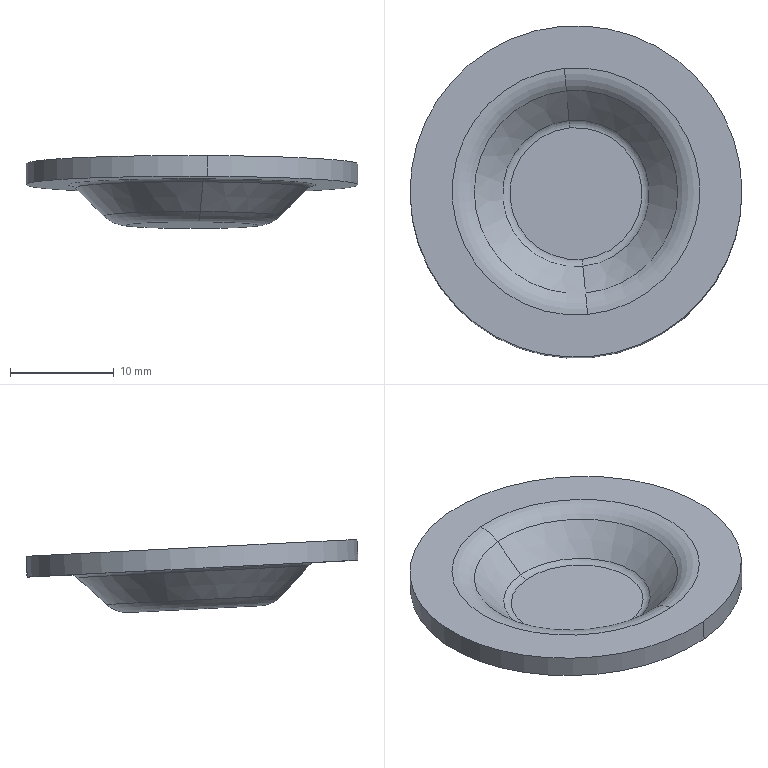Part | SolidWorks | features BaseBody 1 | 1 solid | 18 faces | box 31.952 x 32.01 x 7.031 mm | volume 1769 mm3 | torus 8 | plane 4 | cone 4 | cylinder 2 | commonest cylinder face diameters 31.95 x2
STEP:
#1=CARTESIAN_POINT('',(1922.948,699.088,823.416));
#2=VERTEX_POINT('',#1);
#3=CARTESIAN_POINT('',(1925.951,667.32,825.03));
#4=VERTEX_POINT('',#3);
#5=CARTESIAN_POINT('',(1924.45,683.204,824.223));
#6=DIRECTION('',(0.0008173,0.05081,0.9987));
#7=DIRECTION('',(-0.094,0.9943,-0.05051));
#8=AXIS2_PLACEMENT_3D('',#5,#6,#7);
#9=CIRCLE('',#8,15.975);
#10=EDGE_CURVE('',#2,#4,#9,.T.);
#11=ORIENTED_EDGE('',*,*,#10,.F.);
#12=CARTESIAN_POINT('',(1924.45,683.204,824.223));
#13=DIRECTION('',(-0.0008173,-0.05081,-0.9987));
#14=DIRECTION('',(-0.094,0.9943,-0.05051));
#15=AXIS2_PLACEMENT_3D('',#12,#13,#14);
#16=CIRCLE('',#15,15.975);
#17=EDGE_CURVE('',#2,#4,#16,.T.);
#18=ORIENTED_EDGE('',*,*,#17,.T.);
#19=EDGE_LOOP('',(#11,#18));
#20=FACE_OUTER_BOUND('',#19,.T.);
#21=CARTESIAN_POINT('',(1923.329,695.053,823.621));
#22=VERTEX_POINT('',#21);
#23=CARTESIAN_POINT('',(1925.57,671.354,824.825));
#24=VERTEX_POINT('',#23);
#25=CARTESIAN_POINT('',(1924.45,683.204,824.223));
#26=DIRECTION('',(-0.0008173,-0.05081,-0.9987));
#27=DIRECTION('',(-0.094,0.9943,-0.05051));
#28=AXIS2_PLACEMENT_3D('',#25,#26,#27);
#29=CIRCLE('',#28,11.918);
#30=EDGE_CURVE('',#22,#24,#29,.T.);
#31=ORIENTED_EDGE('',*,*,#30,.F.);
#32=CARTESIAN_POINT('',(1924.45,683.204,824.223));
#33=DIRECTION('',(0.0008173,0.05081,0.9987));
#34=DIRECTION('',(-0.094,0.9943,-0.05051));
#35=AXIS2_PLACEMENT_3D('',#32,#33,#34);
#36=CIRCLE('',#35,11.918);
#37=EDGE_CURVE('',#22,#24,#36,.T.);
#38=ORIENTED_EDGE('',*,*,#37,.T.);
#39=EDGE_LOOP('',(#31,#38));
#40=FACE_BOUND('',#39,.T.);
#41=CARTESIAN_POINT('',(1924.45,683.204,824.223));
#42=DIRECTION('',(0.0008173,0.05081,0.9987));
#43=DIRECTION('',(-0.094,0.9943,-0.05051));
#44=AXIS2_PLACEMENT_3D('',#41,#42,#43);
#45=PLANE('',#44);
#46=ADVANCED_FACE('',(#20,#40),#45,.F.);
#47=CARTESIAN_POINT('',(1923.396,694.335,823.364));
#48=VERTEX_POINT('',#47);
#49=CARTESIAN_POINT('',(1925.503,672.042,824.496));
#50=VERTEX_POINT('',#49);
#51=CARTESIAN_POINT('',(1924.449,683.189,823.93));
#52=DIRECTION('',(0.0008173,0.05081,0.9987));
#53=DIRECTION('',(-0.094,0.9943,-0.05051));
#54=AXIS2_PLACEMENT_3D('',#51,#52,#53);
#55=CIRCLE('',#54,11.211);
#56=EDGE_CURVE('',#48,#50,#55,.T.);
#57=ORIENTED_EDGE('',*,*,#56,.T.);
#58=CARTESIAN_POINT('',(1925.569,671.303,823.826));
#59=DIRECTION('',(-0.9956,-0.09384,0.005589));
#60=DIRECTION('',(0.0008173,0.05081,0.9987));
#61=AXIS2_PLACEMENT_3D('',#58,#59,#60);
#62=CIRCLE('',#61,1.);
#63=EDGE_CURVE('',#24,#50,#62,.T.);
#64=ORIENTED_EDGE('',*,*,#63,.F.);
#65=ORIENTED_EDGE('',*,*,#37,.F.);
#66=CARTESIAN_POINT('',(1923.329,695.003,822.622));
#67=DIRECTION('',(-0.9956,-0.09384,0.005589));
#68=DIRECTION('',(0.0008173,0.05081,0.9987));
#69=AXIS2_PLACEMENT_3D('',#66,#67,#68);
#70=CIRCLE('',#69,1.);
#71=EDGE_CURVE('',#48,#22,#70,.T.);
#72=ORIENTED_EDGE('',*,*,#71,.F.);
#73=EDGE_LOOP('',(#57,#64,#65,#72));
#74=FACE_OUTER_BOUND('',#73,.T.);
#75=CARTESIAN_POINT('',(1924.449,683.153,823.224));
#76=DIRECTION('',(0.0008173,0.05081,0.9987));
#77=DIRECTION('',(-0.094,0.9943,-0.05051));
#78=AXIS2_PLACEMENT_3D('',#75,#76,#77);
#79=TOROIDAL_SURFACE('',#78,11.918,1.);
#80=ADVANCED_FACE('',(#74),#79,.F.);
#81=ORIENTED_EDGE('',*,*,#30,.T.);
#82=ORIENTED_EDGE('',*,*,#63,.T.);
#83=CARTESIAN_POINT('',(1924.449,683.189,823.93));
#84=DIRECTION('',(-0.0008173,-0.05081,-0.9987));
#85=DIRECTION('',(-0.094,0.9943,-0.05051));
#86=AXIS2_PLACEMENT_3D('',#83,#84,#85);
#87=CIRCLE('',#86,11.211);
#88=EDGE_CURVE('',#48,#50,#87,.T.);
#89=ORIENTED_EDGE('',*,*,#88,.F.);
#90=ORIENTED_EDGE('',*,*,#71,.T.);
#91=EDGE_LOOP('',(#81,#82,#89,#90));
#92=FACE_OUTER_BOUND('',#91,.T.);
#93=CARTESIAN_POINT('',(1924.449,683.153,823.224));
#94=DIRECTION('',(0.0008173,0.05081,0.9987));
#95=DIRECTION('',(-0.094,0.9943,-0.05051));
#96=AXIS2_PLACEMENT_3D('',#93,#94,#95);
#97=TOROIDAL_SURFACE('',#96,11.918,1.);
#98=ADVANCED_FACE('',(#92),#97,.F.);
#99=ORIENTED_EDGE('',*,*,#88,.T.);
#100=CARTESIAN_POINT('',(1925.245,674.617,821.634));
#101=VERTEX_POINT('',#100);
#102=CARTESIAN_POINT('',(1925.503,672.042,824.496));
#103=DIRECTION('',(-0.06705,0.6671,-0.7419));
#104=VECTOR('',#103,1000.);
#105=LINE('',#102,#104);
#106=EDGE_CURVE('',#50,#101,#105,.T.);
#107=ORIENTED_EDGE('',*,*,#106,.T.);
#108=CARTESIAN_POINT('',(1923.65,691.484,820.777));
#109=VERTEX_POINT('',#108);
#110=CARTESIAN_POINT('',(1924.447,683.05,821.205));
#111=DIRECTION('',(-0.0008173,-0.05081,-0.9987));
#112=DIRECTION('',(-0.094,0.9943,-0.05051));
#113=AXIS2_PLACEMENT_3D('',#110,#111,#112);
#114=CIRCLE('',#113,8.482);
#115=EDGE_CURVE('',#109,#101,#114,.T.);
#116=ORIENTED_EDGE('',*,*,#115,.F.);
#117=CARTESIAN_POINT('',(1923.396,694.335,823.364));
#118=DIRECTION('',(-0.06589,0.739,0.6705));
#119=VECTOR('',#118,1000.);
#120=LINE('',#117,#119);
#121=EDGE_CURVE('',#109,#48,#120,.T.);
#122=ORIENTED_EDGE('',*,*,#121,.T.);
#123=EDGE_LOOP('',(#99,#107,#116,#122));
#124=FACE_OUTER_BOUND('',#123,.T.);
#125=CARTESIAN_POINT('',(1924.448,683.12,822.568));
#126=DIRECTION('',(0.0008173,0.05081,0.9987));
#127=DIRECTION('',(-0.094,0.9943,-0.05051));
#128=AXIS2_PLACEMENT_3D('',#125,#126,#127);
#129=CONICAL_SURFACE('',#128,9.846,0.7854);
#130=ADVANCED_FACE('',(#124),#129,.T.);
#131=CARTESIAN_POINT('',(1924.447,683.05,821.205));
#132=DIRECTION('',(0.0008173,0.05081,0.9987));
#133=DIRECTION('',(-0.094,0.9943,-0.05051));
#134=AXIS2_PLACEMENT_3D('',#131,#132,#133);
#135=CIRCLE('',#134,8.482);
#136=EDGE_CURVE('',#109,#101,#135,.T.);
#137=ORIENTED_EDGE('',*,*,#136,.T.);
#138=ORIENTED_EDGE('',*,*,#106,.F.);
#139=ORIENTED_EDGE('',*,*,#56,.F.);
#140=ORIENTED_EDGE('',*,*,#121,.F.);
#141=EDGE_LOOP('',(#137,#138,#139,#140));
#142=FACE_OUTER_BOUND('',#141,.T.);
#143=CARTESIAN_POINT('',(1924.448,683.12,822.568));
#144=DIRECTION('',(0.0008173,0.05081,0.9987));
#145=DIRECTION('',(-0.094,0.9943,-0.05051));
#146=AXIS2_PLACEMENT_3D('',#143,#144,#145);
#147=CONICAL_SURFACE('',#146,9.846,0.7854);
#148=ADVANCED_FACE('',(#142),#147,.T.);
#149=CARTESIAN_POINT('',(1923.849,689.33,820.006));
#150=VERTEX_POINT('',#149);
#151=CARTESIAN_POINT('',(1925.044,676.681,820.649));
#152=VERTEX_POINT('',#151);
#153=CARTESIAN_POINT('',(1924.447,683.006,820.328));
#154=DIRECTION('',(0.0008173,0.05081,0.9987));
#155=DIRECTION('',(-0.094,0.9943,-0.05051));
#156=AXIS2_PLACEMENT_3D('',#153,#154,#155);
#157=CIRCLE('',#156,6.361);
#158=EDGE_CURVE('',#150,#152,#157,.T.);
#159=ORIENTED_EDGE('',*,*,#158,.T.);
#160=CARTESIAN_POINT('',(1925.047,676.834,823.645));
#161=DIRECTION('',(-0.9956,-0.09384,0.005589));
#162=DIRECTION('',(0.06589,-0.739,-0.6705));
#163=AXIS2_PLACEMENT_3D('',#160,#161,#162);
#164=CIRCLE('',#163,3.);
#165=EDGE_CURVE('',#152,#101,#164,.T.);
#166=ORIENTED_EDGE('',*,*,#165,.T.);
#167=ORIENTED_EDGE('',*,*,#136,.F.);
#168=CARTESIAN_POINT('',(1923.851,689.483,823.003));
#169=DIRECTION('',(-0.9956,-0.09384,0.005589));
#170=DIRECTION('',(-0.06705,0.6671,-0.7419));
#171=AXIS2_PLACEMENT_3D('',#168,#169,#170);
#172=CIRCLE('',#171,3.);
#173=EDGE_CURVE('',#109,#150,#172,.T.);
#174=ORIENTED_EDGE('',*,*,#173,.T.);
#175=EDGE_LOOP('',(#159,#166,#167,#174));
#176=FACE_OUTER_BOUND('',#175,.T.);
#177=CARTESIAN_POINT('',(1924.449,683.158,823.324));
#178=DIRECTION('',(0.0008173,0.05081,0.9987));
#179=DIRECTION('',(-0.094,0.9943,-0.05051));
#180=AXIS2_PLACEMENT_3D('',#177,#178,#179);
#181=TOROIDAL_SURFACE('',#180,6.361,3.);
#182=ADVANCED_FACE('',(#176),#181,.T.);
#183=ORIENTED_EDGE('',*,*,#115,.T.);
#184=ORIENTED_EDGE('',*,*,#165,.F.);
#185=CARTESIAN_POINT('',(1924.447,683.006,820.328));
#186=DIRECTION('',(-0.0008173,-0.05081,-0.9987));
#187=DIRECTION('',(-0.094,0.9943,-0.05051));
#188=AXIS2_PLACEMENT_3D('',#185,#186,#187);
#189=CIRCLE('',#188,6.361);
#190=EDGE_CURVE('',#150,#152,#189,.T.);
#191=ORIENTED_EDGE('',*,*,#190,.F.);
#192=ORIENTED_EDGE('',*,*,#173,.F.);
#193=EDGE_LOOP('',(#183,#184,#191,#192));
#194=FACE_OUTER_BOUND('',#193,.T.);
#195=CARTESIAN_POINT('',(1924.449,683.158,823.324));
#196=DIRECTION('',(0.0008173,0.05081,0.9987));
#197=DIRECTION('',(-0.094,0.9943,-0.05051));
#198=AXIS2_PLACEMENT_3D('',#195,#196,#197);
#199=TOROIDAL_SURFACE('',#198,6.361,3.);
#200=ADVANCED_FACE('',(#194),#199,.T.);
#201=ORIENTED_EDGE('',*,*,#158,.F.);
#202=ORIENTED_EDGE('',*,*,#190,.T.);
#203=EDGE_LOOP('',(#201,#202));
#204=FACE_OUTER_BOUND('',#203,.T.);
#205=CARTESIAN_POINT('',(1924.447,683.006,820.328));
#206=DIRECTION('',(0.0008173,0.05081,0.9987));
#207=DIRECTION('',(-0.094,0.9943,-0.05051));
#208=AXIS2_PLACEMENT_3D('',#205,#206,#207);
#209=PLANE('',#208);
#210=ADVANCED_FACE('',(#204),#209,.F.);
#211=CARTESIAN_POINT('',(1922.95,699.189,825.413));
#212=VERTEX_POINT('',#211);
#213=CARTESIAN_POINT('',(1925.953,667.422,827.027));
#214=VERTEX_POINT('',#213);
#215=CARTESIAN_POINT('',(1924.451,683.305,826.22));
#216=DIRECTION('',(-0.0008173,-0.05081,-0.9987));
#217=DIRECTION('',(-0.094,0.9943,-0.05051));
#218=AXIS2_PLACEMENT_3D('',#215,#216,#217);
#219=CIRCLE('',#218,15.975);
#220=EDGE_CURVE('',#212,#214,#219,.T.);
#221=ORIENTED_EDGE('',*,*,#220,.T.);
#222=CARTESIAN_POINT('',(1925.953,667.422,827.027));
#223=DIRECTION('',(-0.0008173,-0.05081,-0.9987));
#224=VECTOR('',#223,1000.);
#225=LINE('',#222,#224);
#226=EDGE_CURVE('',#214,#4,#225,.T.);
#227=ORIENTED_EDGE('',*,*,#226,.T.);
#228=ORIENTED_EDGE('',*,*,#17,.F.);
#229=CARTESIAN_POINT('',(1922.95,699.189,825.413));
#230=DIRECTION('',(0.0008173,0.05081,0.9987));
#231=VECTOR('',#230,1000.);
#232=LINE('',#229,#231);
#233=EDGE_CURVE('',#2,#212,#232,.T.);
#234=ORIENTED_EDGE('',*,*,#233,.T.);
#235=EDGE_LOOP('',(#221,#227,#228,#234));
#236=FACE_OUTER_BOUND('',#235,.T.);
#237=CARTESIAN_POINT('',(1924.446,682.991,820.033));
#238=DIRECTION('',(0.0008173,0.05081,0.9987));
#239=DIRECTION('',(-0.094,0.9943,-0.05051));
#240=AXIS2_PLACEMENT_3D('',#237,#238,#239);
#241=CYLINDRICAL_SURFACE('',#240,15.975);
#242=ADVANCED_FACE('',(#236),#241,.T.);
#243=ORIENTED_EDGE('',*,*,#10,.T.);
#244=ORIENTED_EDGE('',*,*,#226,.F.);
#245=CARTESIAN_POINT('',(1924.451,683.305,826.22));
#246=DIRECTION('',(0.0008173,0.05081,0.9987));
#247=DIRECTION('',(-0.094,0.9943,-0.05051));
#248=AXIS2_PLACEMENT_3D('',#245,#246,#247);
#249=CIRCLE('',#248,15.975);
#250=EDGE_CURVE('',#212,#214,#249,.T.);
#251=ORIENTED_EDGE('',*,*,#250,.F.);
#252=ORIENTED_EDGE('',*,*,#233,.F.);
#253=EDGE_LOOP('',(#243,#244,#251,#252));
#254=FACE_OUTER_BOUND('',#253,.T.);
#255=CARTESIAN_POINT('',(1924.446,682.991,820.033));
#256=DIRECTION('',(0.0008173,0.05081,0.9987));
#257=DIRECTION('',(-0.094,0.9943,-0.05051));
#258=AXIS2_PLACEMENT_3D('',#255,#256,#257);
#259=CYLINDRICAL_SURFACE('',#258,15.975);
#260=ADVANCED_FACE('',(#254),#259,.T.);
#261=ORIENTED_EDGE('',*,*,#250,.T.);
#262=ORIENTED_EDGE('',*,*,#220,.F.);
#263=EDGE_LOOP('',(#261,#262));
#264=FACE_OUTER_BOUND('',#263,.T.);
#265=CARTESIAN_POINT('',(1923.331,695.155,825.618));
#266=VERTEX_POINT('',#265);
#267=CARTESIAN_POINT('',(1925.572,671.456,826.822));
#268=VERTEX_POINT('',#267);
#269=CARTESIAN_POINT('',(1924.451,683.305,826.22));
#270=DIRECTION('',(-0.0008173,-0.05081,-0.9987));
#271=DIRECTION('',(-0.094,0.9943,-0.05051));
#272=AXIS2_PLACEMENT_3D('',#269,#270,#271);
#273=CIRCLE('',#272,11.918);
#274=EDGE_CURVE('',#266,#268,#273,.T.);
#275=ORIENTED_EDGE('',*,*,#274,.T.);
#276=CARTESIAN_POINT('',(1924.451,683.305,826.22));
#277=DIRECTION('',(0.0008173,0.05081,0.9987));
#278=DIRECTION('',(-0.094,0.9943,-0.05051));
#279=AXIS2_PLACEMENT_3D('',#276,#277,#278);
#280=CIRCLE('',#279,11.918);
#281=EDGE_CURVE('',#266,#268,#280,.T.);
#282=ORIENTED_EDGE('',*,*,#281,.F.);
#283=EDGE_LOOP('',(#275,#282));
#284=FACE_BOUND('',#283,.T.);
#285=CARTESIAN_POINT('',(1924.451,683.305,826.22));
#286=DIRECTION('',(0.0008173,0.05081,0.9987));
#287=DIRECTION('',(-0.094,0.9943,-0.05051));
#288=AXIS2_PLACEMENT_3D('',#285,#286,#287);
#289=PLANE('',#288);
#290=ADVANCED_FACE('',(#264,#284),#289,.T.);
#291=ORIENTED_EDGE('',*,*,#281,.T.);
#292=CARTESIAN_POINT('',(1925.372,673.52,825.837));
#293=VERTEX_POINT('',#292);
#294=CARTESIAN_POINT('',(1925.569,671.303,823.826));
#295=DIRECTION('',(-0.9956,-0.09384,0.005589));
#296=DIRECTION('',(-0.06589,0.739,0.6705));
#297=AXIS2_PLACEMENT_3D('',#294,#295,#296);
#298=CIRCLE('',#297,3.);
#299=EDGE_CURVE('',#268,#293,#298,.T.);
#300=ORIENTED_EDGE('',*,*,#299,.T.);
#301=CARTESIAN_POINT('',(1923.53,693.001,824.848));
#302=VERTEX_POINT('',#301);
#303=CARTESIAN_POINT('',(1924.451,683.261,825.343));
#304=DIRECTION('',(0.0008173,0.05081,0.9987));
#305=DIRECTION('',(-0.094,0.9943,-0.05051));
#306=AXIS2_PLACEMENT_3D('',#303,#304,#305);
#307=CIRCLE('',#306,9.796);
#308=EDGE_CURVE('',#302,#293,#307,.T.);
#309=ORIENTED_EDGE('',*,*,#308,.F.);
#310=CARTESIAN_POINT('',(1923.329,695.003,822.622));
#311=DIRECTION('',(-0.9956,-0.09384,0.005589));
#312=DIRECTION('',(0.06705,-0.6671,0.7419));
#313=AXIS2_PLACEMENT_3D('',#310,#311,#312);
#314=CIRCLE('',#313,3.);
#315=EDGE_CURVE('',#302,#266,#314,.T.);
#316=ORIENTED_EDGE('',*,*,#315,.T.);
#317=EDGE_LOOP('',(#291,#300,#309,#316));
#318=FACE_OUTER_BOUND('',#317,.T.);
#319=CARTESIAN_POINT('',(1924.449,683.153,823.224));
#320=DIRECTION('',(0.0008173,0.05081,0.9987));
#321=DIRECTION('',(-0.094,0.9943,-0.05051));
#322=AXIS2_PLACEMENT_3D('',#319,#320,#321);
#323=TOROIDAL_SURFACE('',#322,11.918,3.);
#324=ADVANCED_FACE('',(#318),#323,.T.);
#325=CARTESIAN_POINT('',(1924.451,683.261,825.343));
#326=DIRECTION('',(-0.0008173,-0.05081,-0.9987));
#327=DIRECTION('',(-0.094,0.9943,-0.05051));
#328=AXIS2_PLACEMENT_3D('',#325,#326,#327);
#329=CIRCLE('',#328,9.796);
#330=EDGE_CURVE('',#302,#293,#329,.T.);
#331=ORIENTED_EDGE('',*,*,#330,.T.);
#332=ORIENTED_EDGE('',*,*,#299,.F.);
#333=ORIENTED_EDGE('',*,*,#274,.F.);
#334=ORIENTED_EDGE('',*,*,#315,.F.);
#335=EDGE_LOOP('',(#331,#332,#333,#334));
#336=FACE_OUTER_BOUND('',#335,.T.);
#337=CARTESIAN_POINT('',(1924.449,683.153,823.224));
#338=DIRECTION('',(0.0008173,0.05081,0.9987));
#339=DIRECTION('',(-0.094,0.9943,-0.05051));
#340=AXIS2_PLACEMENT_3D('',#337,#338,#339);
#341=TOROIDAL_SURFACE('',#340,11.918,3.);
#342=ADVANCED_FACE('',(#336),#341,.T.);
#343=CARTESIAN_POINT('',(1923.784,690.15,822.261));
#344=VERTEX_POINT('',#343);
#345=CARTESIAN_POINT('',(1925.113,676.095,822.975));
#346=VERTEX_POINT('',#345);
#347=CARTESIAN_POINT('',(1924.448,683.122,822.618));
#348=DIRECTION('',(-0.0008173,-0.05081,-0.9987));
#349=DIRECTION('',(-0.094,0.9943,-0.05051));
#350=AXIS2_PLACEMENT_3D('',#347,#348,#349);
#351=CIRCLE('',#350,7.068);
#352=EDGE_CURVE('',#344,#346,#351,.T.);
#353=ORIENTED_EDGE('',*,*,#352,.T.);
#354=CARTESIAN_POINT('',(1925.113,676.095,822.975));
#355=DIRECTION('',(-0.06705,0.6671,-0.7419));
#356=VECTOR('',#355,1000.);
#357=LINE('',#354,#356);
#358=EDGE_CURVE('',#293,#346,#357,.T.);
#359=ORIENTED_EDGE('',*,*,#358,.F.);
#360=ORIENTED_EDGE('',*,*,#330,.F.);
#361=CARTESIAN_POINT('',(1923.784,690.15,822.261));
#362=DIRECTION('',(-0.06589,0.739,0.6705));
#363=VECTOR('',#362,1000.);
#364=LINE('',#361,#363);
#365=EDGE_CURVE('',#344,#302,#364,.T.);
#366=ORIENTED_EDGE('',*,*,#365,.F.);
#367=EDGE_LOOP('',(#353,#359,#360,#366));
#368=FACE_OUTER_BOUND('',#367,.T.);
#369=CARTESIAN_POINT('',(1924.45,683.191,823.98));
#370=DIRECTION('',(0.0008173,0.05081,0.9987));
#371=DIRECTION('',(-0.094,0.9943,-0.05051));
#372=AXIS2_PLACEMENT_3D('',#369,#370,#371);
#373=CONICAL_SURFACE('',#372,8.432,0.7854);
#374=ADVANCED_FACE('',(#368),#373,.F.);
#375=ORIENTED_EDGE('',*,*,#308,.T.);
#376=ORIENTED_EDGE('',*,*,#358,.T.);
#377=CARTESIAN_POINT('',(1924.448,683.122,822.618));
#378=DIRECTION('',(0.0008173,0.05081,0.9987));
#379=DIRECTION('',(-0.094,0.9943,-0.05051));
#380=AXIS2_PLACEMENT_3D('',#377,#378,#379);
#381=CIRCLE('',#380,7.068);
#382=EDGE_CURVE('',#344,#346,#381,.T.);
#383=ORIENTED_EDGE('',*,*,#382,.F.);
#384=ORIENTED_EDGE('',*,*,#365,.T.);
#385=EDGE_LOOP('',(#375,#376,#383,#384));
#386=FACE_OUTER_BOUND('',#385,.T.);
#387=CARTESIAN_POINT('',(1924.45,683.191,823.98));
#388=DIRECTION('',(0.0008173,0.05081,0.9987));
#389=DIRECTION('',(-0.094,0.9943,-0.05051));
#390=AXIS2_PLACEMENT_3D('',#387,#388,#389);
#391=CONICAL_SURFACE('',#390,8.432,0.7854);
#392=ADVANCED_FACE('',(#386),#391,.F.);
#393=ORIENTED_EDGE('',*,*,#382,.T.);
#394=CARTESIAN_POINT('',(1925.046,676.783,822.646));
#395=VERTEX_POINT('',#394);
#396=CARTESIAN_POINT('',(1925.047,676.834,823.645));
#397=DIRECTION('',(0.9956,0.09384,-0.005589));
#398=DIRECTION('',(-0.0008173,-0.05081,-0.9987));
#399=AXIS2_PLACEMENT_3D('',#396,#397,#398);
#400=CIRCLE('',#399,1.);
#401=EDGE_CURVE('',#346,#395,#400,.T.);
#402=ORIENTED_EDGE('',*,*,#401,.T.);
#403=CARTESIAN_POINT('',(1923.85,689.432,822.004));
#404=VERTEX_POINT('',#403);
#405=CARTESIAN_POINT('',(1924.448,683.107,822.325));
#406=DIRECTION('',(0.0008173,0.05081,0.9987));
#407=DIRECTION('',(-0.094,0.9943,-0.05051));
#408=AXIS2_PLACEMENT_3D('',#405,#406,#407);
#409=CIRCLE('',#408,6.361);
#410=EDGE_CURVE('',#404,#395,#409,.T.);
#411=ORIENTED_EDGE('',*,*,#410,.F.);
#412=CARTESIAN_POINT('',(1923.851,689.483,823.003));
#413=DIRECTION('',(0.9956,0.09384,-0.005589));
#414=DIRECTION('',(-0.0008173,-0.05081,-0.9987));
#415=AXIS2_PLACEMENT_3D('',#412,#413,#414);
#416=CIRCLE('',#415,1.);
#417=EDGE_CURVE('',#404,#344,#416,.T.);
#418=ORIENTED_EDGE('',*,*,#417,.T.);
#419=EDGE_LOOP('',(#393,#402,#411,#418));
#420=FACE_OUTER_BOUND('',#419,.T.);
#421=CARTESIAN_POINT('',(1924.449,683.158,823.324));
#422=DIRECTION('',(0.0008173,0.05081,0.9987));
#423=DIRECTION('',(-0.094,0.9943,-0.05051));
#424=AXIS2_PLACEMENT_3D('',#421,#422,#423);
#425=TOROIDAL_SURFACE('',#424,6.361,1.);
#426=ADVANCED_FACE('',(#420),#425,.F.);
#427=CARTESIAN_POINT('',(1924.448,683.107,822.325));
#428=DIRECTION('',(-0.0008173,-0.05081,-0.9987));
#429=DIRECTION('',(-0.094,0.9943,-0.05051));
#430=AXIS2_PLACEMENT_3D('',#427,#428,#429);
#431=CIRCLE('',#430,6.361);
#432=EDGE_CURVE('',#404,#395,#431,.T.);
#433=ORIENTED_EDGE('',*,*,#432,.T.);
#434=ORIENTED_EDGE('',*,*,#401,.F.);
#435=ORIENTED_EDGE('',*,*,#352,.F.);
#436=ORIENTED_EDGE('',*,*,#417,.F.);
#437=EDGE_LOOP('',(#433,#434,#435,#436));
#438=FACE_OUTER_BOUND('',#437,.T.);
#439=CARTESIAN_POINT('',(1924.449,683.158,823.324));
#440=DIRECTION('',(0.0008173,0.05081,0.9987));
#441=DIRECTION('',(-0.094,0.9943,-0.05051));
#442=AXIS2_PLACEMENT_3D('',#439,#440,#441);
#443=TOROIDAL_SURFACE('',#442,6.361,1.);
#444=ADVANCED_FACE('',(#438),#443,.F.);
#445=ORIENTED_EDGE('',*,*,#410,.T.);
#446=ORIENTED_EDGE('',*,*,#432,.F.);
#447=EDGE_LOOP('',(#445,#446));
#448=FACE_OUTER_BOUND('',#447,.T.);
#449=CARTESIAN_POINT('',(1924.448,683.107,822.325));
#450=DIRECTION('',(0.0008173,0.05081,0.9987));
#451=DIRECTION('',(-0.094,0.9943,-0.05051));
#452=AXIS2_PLACEMENT_3D('',#449,#450,#451);
#453=PLANE('',#452);
#454=ADVANCED_FACE('',(#448),#453,.T.);
#455=CLOSED_SHELL('',(#46,#80,#98,#130,#148,#182,#200,#210,#242,#260,#290,#324,#342,#374,#392,#426,#444,#454));
#456=MANIFOLD_SOLID_BREP('',#455);
#457=CARTESIAN_POINT('',(0.,0.,0.));
#458=DIRECTION('',(0.,0.,1.));
#459=DIRECTION('',(1.,0.,0.));
#460=AXIS2_PLACEMENT_3D('',#457,#458,#459);
#461=(LENGTH_UNIT()NAMED_UNIT(*)SI_UNIT(.MILLI.,.METRE.));
#462=UNCERTAINTY_MEASURE_WITH_UNIT(LENGTH_MEASURE(0.00001),#461,'','');
#463=(NAMED_UNIT(*)PLANE_ANGLE_UNIT()SI_UNIT($,.RADIAN.));
#464=(NAMED_UNIT(*)SI_UNIT($,.STERADIAN.)SOLID_ANGLE_UNIT());
#465=(GEOMETRIC_REPRESENTATION_CONTEXT(3)GLOBAL_UNCERTAINTY_ASSIGNED_CONTEXT((#462))GLOBAL_UNIT_ASSIGNED_CONTEXT((#461,#463,#464))REPRESENTATION_CONTEXT('',''));
#466=ADVANCED_BREP_SHAPE_REPRESENTATION('',(#456,#460),#465);